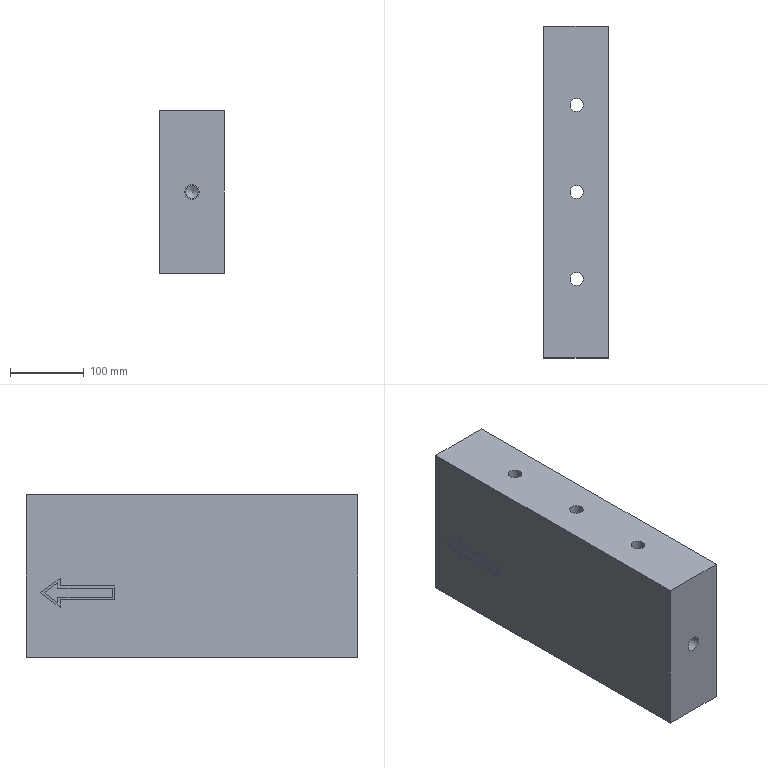Part | STEP file | CC02 | 1 solid | 37 faces | box 88 x 450 x 220 mm | volume 8509495 mm3 | plane 19 | cylinder 9 | spline 5 | cone 4 | commonest cylinder face diameters 18 x3 12 x2 17.4 x2 20 x2